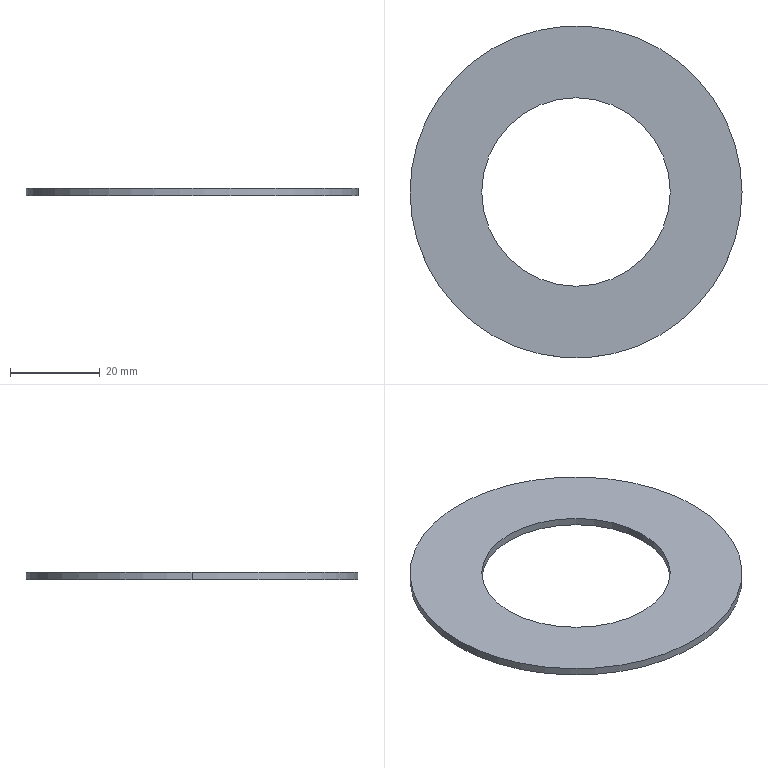Part | SolidWorks | features Extrusion 1 | 1 solid | 6 faces | box 74 x 74 x 1.71 mm | volume 4985 mm3 | cylinder 4 | plane 2 | commonest cylinder face diameters 42 x2 74 x2
STEP:
#1=CARTESIAN_POINT('',(21.,0.,1.71));
#2=VERTEX_POINT('',#1);
#3=CARTESIAN_POINT('',(-21.,0.,1.71));
#4=VERTEX_POINT('',#3);
#5=CARTESIAN_POINT('',(0.,0.,1.71));
#6=DIRECTION('',(0.,0.,-1.));
#7=DIRECTION('',(0.,1.,0.));
#8=AXIS2_PLACEMENT_3D('',#5,#6,#7);
#9=CIRCLE('',#8,21.);
#10=EDGE_CURVE('',#2,#4,#9,.T.);
#11=ORIENTED_EDGE('',*,*,#10,.F.);
#12=CARTESIAN_POINT('',(21.,0.,0.));
#13=VERTEX_POINT('',#12);
#14=CARTESIAN_POINT('',(21.,0.,106.362));
#15=DIRECTION('',(0.,0.,-1.));
#16=VECTOR('',#15,1000.);
#17=LINE('',#14,#16);
#18=EDGE_CURVE('',#2,#13,#17,.T.);
#19=ORIENTED_EDGE('',*,*,#18,.T.);
#20=CARTESIAN_POINT('',(-21.,0.,0.));
#21=VERTEX_POINT('',#20);
#22=CARTESIAN_POINT('',(0.,0.,0.));
#23=DIRECTION('',(0.,0.,1.));
#24=DIRECTION('',(1.,0.,0.));
#25=AXIS2_PLACEMENT_3D('',#22,#23,#24);
#26=CIRCLE('',#25,21.);
#27=EDGE_CURVE('',#21,#13,#26,.T.);
#28=ORIENTED_EDGE('',*,*,#27,.F.);
#29=CARTESIAN_POINT('',(-21.,0.,106.362));
#30=DIRECTION('',(0.,0.,-1.));
#31=VECTOR('',#30,1000.);
#32=LINE('',#29,#31);
#33=EDGE_CURVE('',#4,#21,#32,.T.);
#34=ORIENTED_EDGE('',*,*,#33,.F.);
#35=EDGE_LOOP('',(#11,#19,#28,#34));
#36=FACE_OUTER_BOUND('',#35,.T.);
#37=CARTESIAN_POINT('',(0.,0.,106.362));
#38=DIRECTION('',(0.,0.,-1.));
#39=DIRECTION('',(-1.,0.,0.));
#40=AXIS2_PLACEMENT_3D('',#37,#38,#39);
#41=CYLINDRICAL_SURFACE('',#40,21.);
#42=ADVANCED_FACE('',(#36),#41,.F.);
#43=CARTESIAN_POINT('',(-37.,0.,1.71));
#44=VERTEX_POINT('',#43);
#45=CARTESIAN_POINT('',(37.,0.,1.71));
#46=VERTEX_POINT('',#45);
#47=CARTESIAN_POINT('',(0.,0.,1.71));
#48=DIRECTION('',(0.,0.,-1.));
#49=DIRECTION('',(0.,1.,0.));
#50=AXIS2_PLACEMENT_3D('',#47,#48,#49);
#51=CIRCLE('',#50,37.);
#52=EDGE_CURVE('',#44,#46,#51,.T.);
#53=ORIENTED_EDGE('',*,*,#52,.T.);
#54=CARTESIAN_POINT('',(37.,0.,0.));
#55=VERTEX_POINT('',#54);
#56=CARTESIAN_POINT('',(37.,0.,106.362));
#57=DIRECTION('',(0.,0.,-1.));
#58=VECTOR('',#57,1000.);
#59=LINE('',#56,#58);
#60=EDGE_CURVE('',#46,#55,#59,.T.);
#61=ORIENTED_EDGE('',*,*,#60,.T.);
#62=CARTESIAN_POINT('',(-37.,0.,0.));
#63=VERTEX_POINT('',#62);
#64=CARTESIAN_POINT('',(0.,0.,0.));
#65=DIRECTION('',(0.,0.,1.));
#66=DIRECTION('',(1.,0.,0.));
#67=AXIS2_PLACEMENT_3D('',#64,#65,#66);
#68=CIRCLE('',#67,37.);
#69=EDGE_CURVE('',#55,#63,#68,.T.);
#70=ORIENTED_EDGE('',*,*,#69,.T.);
#71=CARTESIAN_POINT('',(-37.,0.,106.362));
#72=DIRECTION('',(0.,0.,-1.));
#73=VECTOR('',#72,1000.);
#74=LINE('',#71,#73);
#75=EDGE_CURVE('',#44,#63,#74,.T.);
#76=ORIENTED_EDGE('',*,*,#75,.F.);
#77=EDGE_LOOP('',(#53,#61,#70,#76));
#78=FACE_OUTER_BOUND('',#77,.T.);
#79=CARTESIAN_POINT('',(0.,0.,106.362));
#80=DIRECTION('',(0.,0.,-1.));
#81=DIRECTION('',(-1.,0.,0.));
#82=AXIS2_PLACEMENT_3D('',#79,#80,#81);
#83=CYLINDRICAL_SURFACE('',#82,37.);
#84=ADVANCED_FACE('',(#78),#83,.T.);
#85=CARTESIAN_POINT('',(0.,0.,0.));
#86=DIRECTION('',(0.,0.,1.));
#87=DIRECTION('',(1.,0.,0.));
#88=AXIS2_PLACEMENT_3D('',#85,#86,#87);
#89=CIRCLE('',#88,37.);
#90=EDGE_CURVE('',#63,#55,#89,.T.);
#91=ORIENTED_EDGE('',*,*,#90,.F.);
#92=ORIENTED_EDGE('',*,*,#69,.F.);
#93=EDGE_LOOP('',(#91,#92));
#94=FACE_OUTER_BOUND('',#93,.T.);
#95=ORIENTED_EDGE('',*,*,#27,.T.);
#96=CARTESIAN_POINT('',(0.,0.,0.));
#97=DIRECTION('',(0.,0.,1.));
#98=DIRECTION('',(1.,0.,0.));
#99=AXIS2_PLACEMENT_3D('',#96,#97,#98);
#100=CIRCLE('',#99,21.);
#101=EDGE_CURVE('',#13,#21,#100,.T.);
#102=ORIENTED_EDGE('',*,*,#101,.T.);
#103=EDGE_LOOP('',(#95,#102));
#104=FACE_BOUND('',#103,.T.);
#105=CARTESIAN_POINT('',(0.,0.,0.));
#106=DIRECTION('',(0.,0.,1.));
#107=DIRECTION('',(1.,0.,0.));
#108=AXIS2_PLACEMENT_3D('',#105,#106,#107);
#109=PLANE('',#108);
#110=ADVANCED_FACE('',(#94,#104),#109,.F.);
#111=ORIENTED_EDGE('',*,*,#60,.F.);
#112=CARTESIAN_POINT('',(0.,0.,1.71));
#113=DIRECTION('',(0.,0.,-1.));
#114=DIRECTION('',(0.,1.,0.));
#115=AXIS2_PLACEMENT_3D('',#112,#113,#114);
#116=CIRCLE('',#115,37.);
#117=EDGE_CURVE('',#46,#44,#116,.T.);
#118=ORIENTED_EDGE('',*,*,#117,.T.);
#119=ORIENTED_EDGE('',*,*,#75,.T.);
#120=ORIENTED_EDGE('',*,*,#90,.T.);
#121=EDGE_LOOP('',(#111,#118,#119,#120));
#122=FACE_OUTER_BOUND('',#121,.T.);
#123=CARTESIAN_POINT('',(0.,0.,106.362));
#124=DIRECTION('',(0.,0.,-1.));
#125=DIRECTION('',(-1.,0.,0.));
#126=AXIS2_PLACEMENT_3D('',#123,#124,#125);
#127=CYLINDRICAL_SURFACE('',#126,37.);
#128=ADVANCED_FACE('',(#122),#127,.T.);
#129=ORIENTED_EDGE('',*,*,#18,.F.);
#130=CARTESIAN_POINT('',(0.,0.,1.71));
#131=DIRECTION('',(0.,0.,-1.));
#132=DIRECTION('',(0.,1.,0.));
#133=AXIS2_PLACEMENT_3D('',#130,#131,#132);
#134=CIRCLE('',#133,21.);
#135=EDGE_CURVE('',#4,#2,#134,.T.);
#136=ORIENTED_EDGE('',*,*,#135,.F.);
#137=ORIENTED_EDGE('',*,*,#33,.T.);
#138=ORIENTED_EDGE('',*,*,#101,.F.);
#139=EDGE_LOOP('',(#129,#136,#137,#138));
#140=FACE_OUTER_BOUND('',#139,.T.);
#141=CARTESIAN_POINT('',(0.,0.,106.362));
#142=DIRECTION('',(0.,0.,-1.));
#143=DIRECTION('',(-1.,0.,0.));
#144=AXIS2_PLACEMENT_3D('',#141,#142,#143);
#145=CYLINDRICAL_SURFACE('',#144,21.);
#146=ADVANCED_FACE('',(#140),#145,.F.);
#147=ORIENTED_EDGE('',*,*,#135,.T.);
#148=ORIENTED_EDGE('',*,*,#10,.T.);
#149=EDGE_LOOP('',(#147,#148));
#150=FACE_BOUND('',#149,.T.);
#151=ORIENTED_EDGE('',*,*,#52,.F.);
#152=ORIENTED_EDGE('',*,*,#117,.F.);
#153=EDGE_LOOP('',(#151,#152));
#154=FACE_OUTER_BOUND('',#153,.T.);
#155=CARTESIAN_POINT('',(0.,37.5,1.71));
#156=DIRECTION('',(0.,0.,-1.));
#157=DIRECTION('',(0.,1.,0.));
#158=AXIS2_PLACEMENT_3D('',#155,#156,#157);
#159=PLANE('',#158);
#160=ADVANCED_FACE('',(#150,#154),#159,.F.);
#161=CLOSED_SHELL('',(#42,#84,#110,#128,#146,#160));
#162=MANIFOLD_SOLID_BREP('',#161);
#163=CARTESIAN_POINT('',(0.,0.,0.));
#164=DIRECTION('',(0.,0.,1.));
#165=DIRECTION('',(1.,0.,0.));
#166=AXIS2_PLACEMENT_3D('',#163,#164,#165);
#167=(LENGTH_UNIT()NAMED_UNIT(*)SI_UNIT(.MILLI.,.METRE.));
#168=UNCERTAINTY_MEASURE_WITH_UNIT(LENGTH_MEASURE(0.00001),#167,'','');
#169=(NAMED_UNIT(*)PLANE_ANGLE_UNIT()SI_UNIT($,.RADIAN.));
#170=(NAMED_UNIT(*)SI_UNIT($,.STERADIAN.)SOLID_ANGLE_UNIT());
#171=(GEOMETRIC_REPRESENTATION_CONTEXT(3)GLOBAL_UNCERTAINTY_ASSIGNED_CONTEXT((#168))GLOBAL_UNIT_ASSIGNED_CONTEXT((#167,#169,#170))REPRESENTATION_CONTEXT('',''));
#172=ADVANCED_BREP_SHAPE_REPRESENTATION('',(#162,#166),#171);